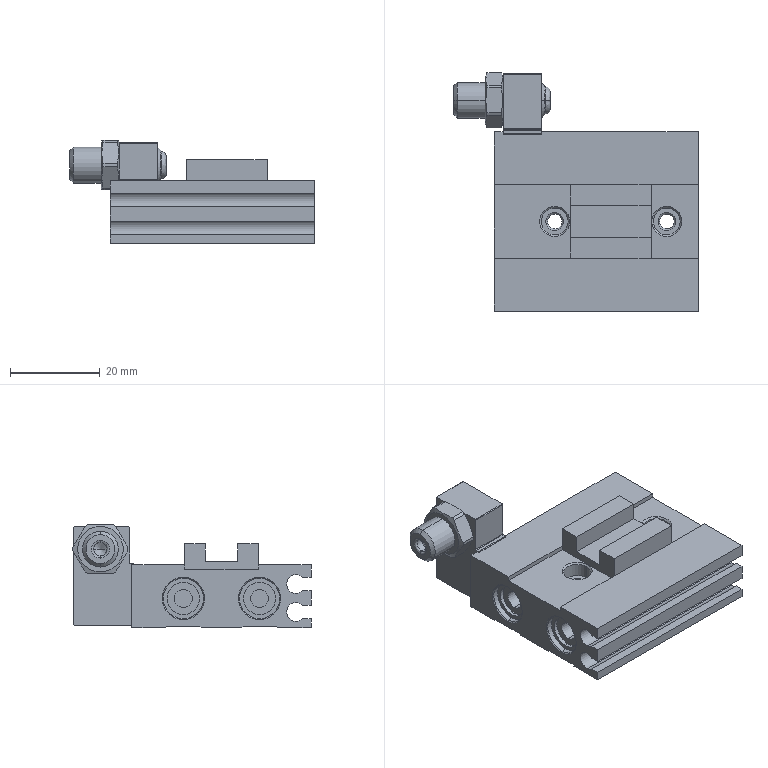Part | STEP file | HLQ8-10-S-AS-1-1 | 1 solid | 254 faces | box 54.5 x 53.15 x 23 mm | volume 23143 mm3 | plane 91 | cylinder 89 | cone 66 | spline 8 | commonest cylinder face diameters 2.459 x12 6 x10 8 x8 9 x8 3 x7 4.2 x6